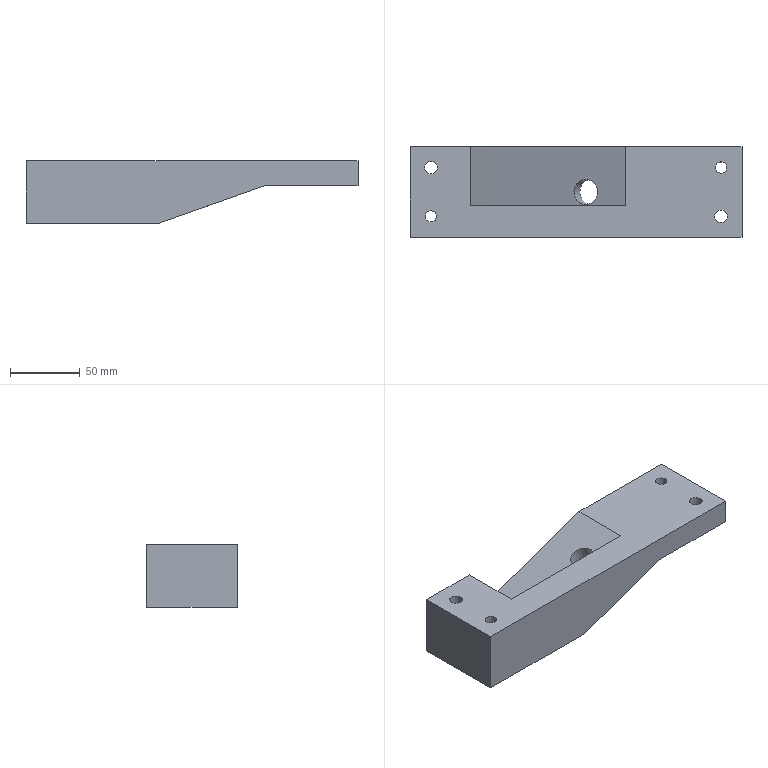Part | STEP file | HYDRAULIC-CYLINDER-BASE1_id474_x_t | 1 solid | 22 faces | box 238 x 65 x 45 mm | volume 410025 mm3 | plane 14 | cylinder 8 | commonest cylinder face diameters 8 x2 9 x2 14 x2 18 x1 31 x1
STEP:
#1=CARTESIAN_POINT('',(70.605,-50.,-302.095));
#2=VERTEX_POINT('',#1);
#3=CARTESIAN_POINT('',(85.215,-50.,-296.921));
#4=DIRECTION('',(0.3338,0.,-0.9426));
#5=DIRECTION('',(-0.9426,0.,-0.3338));
#6=AXIS2_PLACEMENT_3D('',#3,#4,#5);
#7=CIRCLE('',#6,15.5);
#8=EDGE_CURVE('',#2,#2,#7,.T.);
#9=ORIENTED_EDGE('',*,*,#8,.F.);
#10=EDGE_LOOP('',(#9));
#11=FACE_BOUND('',#10,.T.);
#12=CARTESIAN_POINT('',(73.943,-50.,-311.521));
#13=VERTEX_POINT('',#12);
#14=CARTESIAN_POINT('',(88.554,-50.,-306.347));
#15=DIRECTION('',(-0.3338,0.,0.9426));
#16=DIRECTION('',(-0.9426,0.,-0.3338));
#17=AXIS2_PLACEMENT_3D('',#14,#15,#16);
#18=CIRCLE('',#17,15.5);
#19=EDGE_CURVE('',#13,#13,#18,.T.);
#20=ORIENTED_EDGE('',*,*,#19,.F.);
#21=EDGE_LOOP('',(#20));
#22=FACE_BOUND('',#21,.T.);
#23=CARTESIAN_POINT('',(88.554,-50.,-306.347));
#24=DIRECTION('',(0.3338,0.,-0.9426));
#25=DIRECTION('',(-0.9426,0.,-0.3338));
#26=AXIS2_PLACEMENT_3D('',#23,#24,#25);
#27=CYLINDRICAL_SURFACE('',#26,15.5);
#28=ADVANCED_FACE('',(#11,#22),#27,.F.);
#29=CARTESIAN_POINT('',(76.732,-50.,-299.925));
#30=VERTEX_POINT('',#29);
#31=CARTESIAN_POINT('',(85.215,-50.,-296.921));
#32=DIRECTION('',(-0.3338,0.,0.9426));
#33=DIRECTION('',(-0.9426,0.,-0.3338));
#34=AXIS2_PLACEMENT_3D('',#31,#32,#33);
#35=CIRCLE('',#34,9.);
#36=EDGE_CURVE('',#30,#30,#35,.T.);
#37=ORIENTED_EDGE('',*,*,#36,.T.);
#38=EDGE_LOOP('',(#37));
#39=FACE_BOUND('',#38,.T.);
#40=ORIENTED_EDGE('',*,*,#8,.T.);
#41=EDGE_LOOP('',(#40));
#42=FACE_BOUND('',#41,.T.);
#43=CARTESIAN_POINT('',(-161.322,-82.5,-384.224));
#44=DIRECTION('',(0.3338,0.,-0.9426));
#45=DIRECTION('',(-0.9426,0.,-0.3338));
#46=AXIS2_PLACEMENT_3D('',#43,#44,#45);
#47=PLANE('',#46);
#48=ADVANCED_FACE('',(#39,#42),#47,.T.);
#49=CARTESIAN_POINT('',(-37.,-32.5,-311.));
#50=VERTEX_POINT('',#49);
#51=CARTESIAN_POINT('',(-30.,-32.5,-311.));
#52=DIRECTION('',(0.,0.,-1.));
#53=DIRECTION('',(-1.,0.,0.));
#54=AXIS2_PLACEMENT_3D('',#51,#52,#53);
#55=CIRCLE('',#54,7.);
#56=EDGE_CURVE('',#50,#50,#55,.T.);
#57=ORIENTED_EDGE('',*,*,#56,.F.);
#58=EDGE_LOOP('',(#57));
#59=FACE_BOUND('',#58,.T.);
#60=CARTESIAN_POINT('',(-37.,-32.5,-320.));
#61=VERTEX_POINT('',#60);
#62=CARTESIAN_POINT('',(-30.,-32.5,-320.));
#63=DIRECTION('',(0.,0.,1.));
#64=DIRECTION('',(-1.,0.,0.));
#65=AXIS2_PLACEMENT_3D('',#62,#63,#64);
#66=CIRCLE('',#65,7.);
#67=EDGE_CURVE('',#61,#61,#66,.T.);
#68=ORIENTED_EDGE('',*,*,#67,.F.);
#69=EDGE_LOOP('',(#68));
#70=FACE_BOUND('',#69,.T.);
#71=CARTESIAN_POINT('',(-30.,-32.5,-320.));
#72=DIRECTION('',(0.,0.,-1.));
#73=DIRECTION('',(-1.,0.,0.));
#74=AXIS2_PLACEMENT_3D('',#71,#72,#73);
#75=CYLINDRICAL_SURFACE('',#74,7.);
#76=ADVANCED_FACE('',(#59,#70),#75,.F.);
#77=CARTESIAN_POINT('',(171.,-67.5,-284.));
#78=VERTEX_POINT('',#77);
#79=CARTESIAN_POINT('',(178.,-67.5,-284.));
#80=DIRECTION('',(0.,0.,-1.));
#81=DIRECTION('',(-1.,0.,0.));
#82=AXIS2_PLACEMENT_3D('',#79,#80,#81);
#83=CIRCLE('',#82,7.);
#84=EDGE_CURVE('',#78,#78,#83,.T.);
#85=ORIENTED_EDGE('',*,*,#84,.F.);
#86=EDGE_LOOP('',(#85));
#87=FACE_BOUND('',#86,.T.);
#88=CARTESIAN_POINT('',(171.,-67.5,-293.));
#89=VERTEX_POINT('',#88);
#90=CARTESIAN_POINT('',(178.,-67.5,-293.));
#91=DIRECTION('',(0.,0.,1.));
#92=DIRECTION('',(-1.,0.,0.));
#93=AXIS2_PLACEMENT_3D('',#90,#91,#92);
#94=CIRCLE('',#93,7.);
#95=EDGE_CURVE('',#89,#89,#94,.T.);
#96=ORIENTED_EDGE('',*,*,#95,.F.);
#97=EDGE_LOOP('',(#96));
#98=FACE_BOUND('',#97,.T.);
#99=CARTESIAN_POINT('',(178.,-67.5,-293.));
#100=DIRECTION('',(0.,0.,-1.));
#101=DIRECTION('',(-1.,0.,0.));
#102=AXIS2_PLACEMENT_3D('',#99,#100,#101);
#103=CYLINDRICAL_SURFACE('',#102,7.);
#104=ADVANCED_FACE('',(#87,#98),#103,.F.);
#105=ORIENTED_EDGE('',*,*,#19,.T.);
#106=EDGE_LOOP('',(#105));
#107=FACE_BOUND('',#106,.T.);
#108=CARTESIAN_POINT('',(126.246,-82.5,-293.));
#109=VERTEX_POINT('',#108);
#110=CARTESIAN_POINT('',(126.246,-17.5,-293.));
#111=VERTEX_POINT('',#110);
#112=CARTESIAN_POINT('',(126.246,-82.5,-293.));
#113=DIRECTION('',(0.,1.,0.));
#114=VECTOR('',#113,1.);
#115=LINE('',#112,#114);
#116=EDGE_CURVE('',#109,#111,#115,.T.);
#117=ORIENTED_EDGE('',*,*,#116,.F.);
#118=CARTESIAN_POINT('',(50.,-82.5,-320.));
#119=VERTEX_POINT('',#118);
#120=CARTESIAN_POINT('',(126.246,-82.5,-293.));
#121=DIRECTION('',(-0.9426,0.,-0.3338));
#122=VECTOR('',#121,1.);
#123=LINE('',#120,#122);
#124=EDGE_CURVE('',#109,#119,#123,.T.);
#125=ORIENTED_EDGE('',*,*,#124,.T.);
#126=CARTESIAN_POINT('',(50.,-17.5,-320.));
#127=VERTEX_POINT('',#126);
#128=CARTESIAN_POINT('',(50.,-82.5,-320.));
#129=DIRECTION('',(0.,-1.,0.));
#130=VECTOR('',#129,1.);
#131=LINE('',#128,#130);
#132=EDGE_CURVE('',#127,#119,#131,.T.);
#133=ORIENTED_EDGE('',*,*,#132,.F.);
#134=CARTESIAN_POINT('',(126.246,-17.5,-293.));
#135=DIRECTION('',(-0.9426,0.,-0.3338));
#136=VECTOR('',#135,1.);
#137=LINE('',#134,#136);
#138=EDGE_CURVE('',#111,#127,#137,.T.);
#139=ORIENTED_EDGE('',*,*,#138,.F.);
#140=EDGE_LOOP('',(#117,#125,#133,#139));
#141=FACE_BOUND('',#140,.T.);
#142=CARTESIAN_POINT('',(126.246,-82.5,-293.));
#143=DIRECTION('',(0.3338,0.,-0.9426));
#144=DIRECTION('',(-0.9426,0.,-0.3338));
#145=AXIS2_PLACEMENT_3D('',#142,#143,#144);
#146=PLANE('',#145);
#147=ADVANCED_FACE('',(#107,#141),#146,.T.);
#148=ORIENTED_EDGE('',*,*,#36,.F.);
#149=EDGE_LOOP('',(#148));
#150=FACE_BOUND('',#149,.T.);
#151=CARTESIAN_POINT('',(72.541,-50.,-288.092));
#152=VERTEX_POINT('',#151);
#153=CARTESIAN_POINT('',(81.025,-50.,-285.088));
#154=DIRECTION('',(-0.3338,0.,0.9426));
#155=DIRECTION('',(-0.9426,0.,-0.3338));
#156=AXIS2_PLACEMENT_3D('',#153,#154,#155);
#157=CIRCLE('',#156,9.);
#158=EDGE_CURVE('',#152,#152,#157,.T.);
#159=ORIENTED_EDGE('',*,*,#158,.T.);
#160=EDGE_LOOP('',(#159));
#161=FACE_BOUND('',#160,.T.);
#162=CARTESIAN_POINT('',(88.554,-50.,-306.347));
#163=DIRECTION('',(0.3338,0.,-0.9426));
#164=DIRECTION('',(-0.9426,0.,-0.3338));
#165=AXIS2_PLACEMENT_3D('',#162,#163,#164);
#166=CYLINDRICAL_SURFACE('',#165,9.);
#167=ADVANCED_FACE('',(#150,#161),#166,.F.);
#168=CARTESIAN_POINT('',(-34.5,-32.5,-311.));
#169=VERTEX_POINT('',#168);
#170=CARTESIAN_POINT('',(-30.,-32.5,-311.));
#171=DIRECTION('',(0.,0.,1.));
#172=DIRECTION('',(-1.,0.,0.));
#173=AXIS2_PLACEMENT_3D('',#170,#171,#172);
#174=CIRCLE('',#173,4.5);
#175=EDGE_CURVE('',#169,#169,#174,.T.);
#176=ORIENTED_EDGE('',*,*,#175,.T.);
#177=EDGE_LOOP('',(#176));
#178=FACE_BOUND('',#177,.T.);
#179=ORIENTED_EDGE('',*,*,#56,.T.);
#180=EDGE_LOOP('',(#179));
#181=FACE_BOUND('',#180,.T.);
#182=CARTESIAN_POINT('',(-200.,-82.5,-311.));
#183=DIRECTION('',(0.,0.,-1.));
#184=DIRECTION('',(-1.,0.,0.));
#185=AXIS2_PLACEMENT_3D('',#182,#183,#184);
#186=PLANE('',#185);
#187=ADVANCED_FACE('',(#178,#181),#186,.T.);
#188=ORIENTED_EDGE('',*,*,#67,.T.);
#189=EDGE_LOOP('',(#188));
#190=FACE_BOUND('',#189,.T.);
#191=CARTESIAN_POINT('',(-34.,-67.5,-320.));
#192=VERTEX_POINT('',#191);
#193=CARTESIAN_POINT('',(-30.,-67.5,-320.));
#194=DIRECTION('',(0.,0.,1.));
#195=DIRECTION('',(-1.,0.,0.));
#196=AXIS2_PLACEMENT_3D('',#193,#194,#195);
#197=CIRCLE('',#196,4.);
#198=EDGE_CURVE('',#192,#192,#197,.T.);
#199=ORIENTED_EDGE('',*,*,#198,.T.);
#200=EDGE_LOOP('',(#199));
#201=FACE_BOUND('',#200,.T.);
#202=ORIENTED_EDGE('',*,*,#132,.T.);
#203=CARTESIAN_POINT('',(-45.,-82.5,-320.));
#204=VERTEX_POINT('',#203);
#205=CARTESIAN_POINT('',(-200.,-82.5,-320.));
#206=DIRECTION('',(-1.,0.,0.));
#207=VECTOR('',#206,1.);
#208=LINE('',#205,#207);
#209=EDGE_CURVE('',#119,#204,#208,.T.);
#210=ORIENTED_EDGE('',*,*,#209,.T.);
#211=CARTESIAN_POINT('',(-45.,-17.5,-320.));
#212=VERTEX_POINT('',#211);
#213=CARTESIAN_POINT('',(-45.,-82.5,-320.));
#214=DIRECTION('',(0.,-1.,0.));
#215=VECTOR('',#214,1.);
#216=LINE('',#213,#215);
#217=EDGE_CURVE('',#212,#204,#216,.T.);
#218=ORIENTED_EDGE('',*,*,#217,.F.);
#219=CARTESIAN_POINT('',(-200.,-17.5,-320.));
#220=DIRECTION('',(-1.,0.,0.));
#221=VECTOR('',#220,1.);
#222=LINE('',#219,#221);
#223=EDGE_CURVE('',#127,#212,#222,.T.);
#224=ORIENTED_EDGE('',*,*,#223,.F.);
#225=EDGE_LOOP('',(#202,#210,#218,#224));
#226=FACE_BOUND('',#225,.T.);
#227=CARTESIAN_POINT('',(50.,-82.5,-320.));
#228=DIRECTION('',(0.,0.,-1.));
#229=DIRECTION('',(-1.,0.,0.));
#230=AXIS2_PLACEMENT_3D('',#227,#228,#229);
#231=PLANE('',#230);
#232=ADVANCED_FACE('',(#190,#201,#226),#231,.T.);
#233=CARTESIAN_POINT('',(173.5,-67.5,-284.));
#234=VERTEX_POINT('',#233);
#235=CARTESIAN_POINT('',(178.,-67.5,-284.));
#236=DIRECTION('',(0.,0.,1.));
#237=DIRECTION('',(-1.,0.,0.));
#238=AXIS2_PLACEMENT_3D('',#235,#236,#237);
#239=CIRCLE('',#238,4.5);
#240=EDGE_CURVE('',#234,#234,#239,.T.);
#241=ORIENTED_EDGE('',*,*,#240,.T.);
#242=EDGE_LOOP('',(#241));
#243=FACE_BOUND('',#242,.T.);
#244=ORIENTED_EDGE('',*,*,#84,.T.);
#245=EDGE_LOOP('',(#244));
#246=FACE_BOUND('',#245,.T.);
#247=CARTESIAN_POINT('',(-200.,-82.5,-284.));
#248=DIRECTION('',(0.,0.,-1.));
#249=DIRECTION('',(-1.,0.,0.));
#250=AXIS2_PLACEMENT_3D('',#247,#248,#249);
#251=PLANE('',#250);
#252=ADVANCED_FACE('',(#243,#246),#251,.T.);
#253=ORIENTED_EDGE('',*,*,#95,.T.);
#254=EDGE_LOOP('',(#253));
#255=FACE_BOUND('',#254,.T.);
#256=CARTESIAN_POINT('',(174.,-32.5,-293.));
#257=VERTEX_POINT('',#256);
#258=CARTESIAN_POINT('',(178.,-32.5,-293.));
#259=DIRECTION('',(0.,0.,1.));
#260=DIRECTION('',(-1.,0.,0.));
#261=AXIS2_PLACEMENT_3D('',#258,#259,#260);
#262=CIRCLE('',#261,4.);
#263=EDGE_CURVE('',#257,#257,#262,.T.);
#264=ORIENTED_EDGE('',*,*,#263,.T.);
#265=EDGE_LOOP('',(#264));
#266=FACE_BOUND('',#265,.T.);
#267=CARTESIAN_POINT('',(193.,-82.5,-293.));
#268=VERTEX_POINT('',#267);
#269=CARTESIAN_POINT('',(193.,-17.5,-293.));
#270=VERTEX_POINT('',#269);
#271=CARTESIAN_POINT('',(193.,-82.5,-293.));
#272=DIRECTION('',(0.,1.,0.));
#273=VECTOR('',#272,1.);
#274=LINE('',#271,#273);
#275=EDGE_CURVE('',#268,#270,#274,.T.);
#276=ORIENTED_EDGE('',*,*,#275,.F.);
#277=CARTESIAN_POINT('',(-200.,-82.5,-293.));
#278=DIRECTION('',(-1.,0.,0.));
#279=VECTOR('',#278,1.);
#280=LINE('',#277,#279);
#281=EDGE_CURVE('',#268,#109,#280,.T.);
#282=ORIENTED_EDGE('',*,*,#281,.T.);
#283=ORIENTED_EDGE('',*,*,#116,.T.);
#284=CARTESIAN_POINT('',(-200.,-17.5,-293.));
#285=DIRECTION('',(-1.,0.,0.));
#286=VECTOR('',#285,1.);
#287=LINE('',#284,#286);
#288=EDGE_CURVE('',#270,#111,#287,.T.);
#289=ORIENTED_EDGE('',*,*,#288,.F.);
#290=EDGE_LOOP('',(#276,#282,#283,#289));
#291=FACE_BOUND('',#290,.T.);
#292=CARTESIAN_POINT('',(193.,-82.5,-293.));
#293=DIRECTION('',(0.,0.,-1.));
#294=DIRECTION('',(-1.,0.,0.));
#295=AXIS2_PLACEMENT_3D('',#292,#293,#294);
#296=PLANE('',#295);
#297=ADVANCED_FACE('',(#255,#266,#291),#296,.T.);
#298=CARTESIAN_POINT('',(10.798,-60.,-309.957));
#299=VERTEX_POINT('',#298);
#300=CARTESIAN_POINT('',(-1.58,-60.,-275.));
#301=VERTEX_POINT('',#300);
#302=CARTESIAN_POINT('',(10.798,-60.,-309.957));
#303=DIRECTION('',(-0.3338,0.,0.9426));
#304=VECTOR('',#303,1.);
#305=LINE('',#302,#304);
#306=EDGE_CURVE('',#299,#301,#305,.T.);
#307=ORIENTED_EDGE('',*,*,#306,.F.);
#308=CARTESIAN_POINT('',(10.798,-17.5,-309.957));
#309=VERTEX_POINT('',#308);
#310=CARTESIAN_POINT('',(10.798,-17.5,-309.957));
#311=DIRECTION('',(0.,1.,0.));
#312=VECTOR('',#311,1.);
#313=LINE('',#310,#312);
#314=EDGE_CURVE('',#299,#309,#313,.T.);
#315=ORIENTED_EDGE('',*,*,#314,.T.);
#316=CARTESIAN_POINT('',(-1.58,-17.5,-275.));
#317=VERTEX_POINT('',#316);
#318=CARTESIAN_POINT('',(-1.58,-17.5,-275.));
#319=DIRECTION('',(0.3338,0.,-0.9426));
#320=VECTOR('',#319,1.);
#321=LINE('',#318,#320);
#322=EDGE_CURVE('',#317,#309,#321,.T.);
#323=ORIENTED_EDGE('',*,*,#322,.F.);
#324=CARTESIAN_POINT('',(-1.58,-82.5,-275.));
#325=DIRECTION('',(0.,1.,0.));
#326=VECTOR('',#325,1.);
#327=LINE('',#324,#326);
#328=EDGE_CURVE('',#301,#317,#327,.T.);
#329=ORIENTED_EDGE('',*,*,#328,.F.);
#330=EDGE_LOOP('',(#307,#315,#323,#329));
#331=FACE_OUTER_BOUND('',#330,.T.);
#332=CARTESIAN_POINT('',(10.798,-17.5,-309.957));
#333=DIRECTION('',(-0.9426,0.,-0.3338));
#334=DIRECTION('',(-0.3338,0.,0.9426));
#335=AXIS2_PLACEMENT_3D('',#332,#333,#334);
#336=PLANE('',#335);
#337=ADVANCED_FACE('',(#331),#336,.F.);
#338=ORIENTED_EDGE('',*,*,#217,.T.);
#339=CARTESIAN_POINT('',(-45.,-82.5,-275.));
#340=VERTEX_POINT('',#339);
#341=CARTESIAN_POINT('',(-45.,-82.5,-275.));
#342=DIRECTION('',(0.,0.,1.));
#343=VECTOR('',#342,1.);
#344=LINE('',#341,#343);
#345=EDGE_CURVE('',#204,#340,#344,.T.);
#346=ORIENTED_EDGE('',*,*,#345,.T.);
#347=CARTESIAN_POINT('',(-45.,-17.5,-275.));
#348=VERTEX_POINT('',#347);
#349=CARTESIAN_POINT('',(-45.,-82.5,-275.));
#350=DIRECTION('',(0.,-1.,0.));
#351=VECTOR('',#350,1.);
#352=LINE('',#349,#351);
#353=EDGE_CURVE('',#348,#340,#352,.T.);
#354=ORIENTED_EDGE('',*,*,#353,.F.);
#355=CARTESIAN_POINT('',(-45.,-17.5,-275.));
#356=DIRECTION('',(0.,0.,1.));
#357=VECTOR('',#356,1.);
#358=LINE('',#355,#357);
#359=EDGE_CURVE('',#212,#348,#358,.T.);
#360=ORIENTED_EDGE('',*,*,#359,.F.);
#361=EDGE_LOOP('',(#338,#346,#354,#360));
#362=FACE_OUTER_BOUND('',#361,.T.);
#363=CARTESIAN_POINT('',(-45.,-82.5,-320.));
#364=DIRECTION('',(-1.,0.,0.));
#365=DIRECTION('',(0.,0.,1.));
#366=AXIS2_PLACEMENT_3D('',#363,#364,#365);
#367=PLANE('',#366);
#368=ADVANCED_FACE('',(#362),#367,.T.);
#369=ORIENTED_EDGE('',*,*,#124,.F.);
#370=ORIENTED_EDGE('',*,*,#281,.F.);
#371=CARTESIAN_POINT('',(193.,-82.5,-275.));
#372=VERTEX_POINT('',#371);
#373=CARTESIAN_POINT('',(193.,-82.5,-275.));
#374=DIRECTION('',(0.,0.,-1.));
#375=VECTOR('',#374,1.);
#376=LINE('',#373,#375);
#377=EDGE_CURVE('',#372,#268,#376,.T.);
#378=ORIENTED_EDGE('',*,*,#377,.F.);
#379=CARTESIAN_POINT('',(-45.,-82.5,-275.));
#380=DIRECTION('',(1.,0.,0.));
#381=VECTOR('',#380,1.);
#382=LINE('',#379,#381);
#383=EDGE_CURVE('',#340,#372,#382,.T.);
#384=ORIENTED_EDGE('',*,*,#383,.F.);
#385=ORIENTED_EDGE('',*,*,#345,.F.);
#386=ORIENTED_EDGE('',*,*,#209,.F.);
#387=EDGE_LOOP('',(#369,#370,#378,#384,#385,#386));
#388=FACE_OUTER_BOUND('',#387,.T.);
#389=CARTESIAN_POINT('',(-200.,-82.5,-275.));
#390=DIRECTION('',(0.,1.,0.));
#391=DIRECTION('',(0.,0.,1.));
#392=AXIS2_PLACEMENT_3D('',#389,#390,#391);
#393=PLANE('',#392);
#394=ADVANCED_FACE('',(#388),#393,.F.);
#395=CARTESIAN_POINT('',(193.,-17.5,-275.));
#396=VERTEX_POINT('',#395);
#397=CARTESIAN_POINT('',(193.,-82.5,-275.));
#398=DIRECTION('',(0.,1.,0.));
#399=VECTOR('',#398,1.);
#400=LINE('',#397,#399);
#401=EDGE_CURVE('',#372,#396,#400,.T.);
#402=ORIENTED_EDGE('',*,*,#401,.F.);
#403=ORIENTED_EDGE('',*,*,#377,.T.);
#404=ORIENTED_EDGE('',*,*,#275,.T.);
#405=CARTESIAN_POINT('',(193.,-17.5,-275.));
#406=DIRECTION('',(0.,0.,-1.));
#407=VECTOR('',#406,1.);
#408=LINE('',#405,#407);
#409=EDGE_CURVE('',#396,#270,#408,.T.);
#410=ORIENTED_EDGE('',*,*,#409,.F.);
#411=EDGE_LOOP('',(#402,#403,#404,#410));
#412=FACE_OUTER_BOUND('',#411,.T.);
#413=CARTESIAN_POINT('',(193.,-82.5,-275.));
#414=DIRECTION('',(1.,0.,0.));
#415=DIRECTION('',(0.,0.,-1.));
#416=AXIS2_PLACEMENT_3D('',#413,#414,#415);
#417=PLANE('',#416);
#418=ADVANCED_FACE('',(#412),#417,.T.);
#419=CARTESIAN_POINT('',(-45.,-17.5,-275.));
#420=DIRECTION('',(-1.,0.,0.));
#421=VECTOR('',#420,1.);
#422=LINE('',#419,#421);
#423=EDGE_CURVE('',#317,#348,#422,.T.);
#424=ORIENTED_EDGE('',*,*,#423,.F.);
#425=ORIENTED_EDGE('',*,*,#322,.T.);
#426=CARTESIAN_POINT('',(109.513,-17.5,-275.));
#427=VERTEX_POINT('',#426);
#428=CARTESIAN_POINT('',(109.513,-17.5,-275.));
#429=DIRECTION('',(0.9426,0.,0.3338));
#430=VECTOR('',#429,1.);
#431=LINE('',#428,#430);
#432=EDGE_CURVE('',#309,#427,#431,.T.);
#433=ORIENTED_EDGE('',*,*,#432,.T.);
#434=CARTESIAN_POINT('',(-45.,-17.5,-275.));
#435=DIRECTION('',(-1.,0.,0.));
#436=VECTOR('',#435,1.);
#437=LINE('',#434,#436);
#438=EDGE_CURVE('',#396,#427,#437,.T.);
#439=ORIENTED_EDGE('',*,*,#438,.F.);
#440=ORIENTED_EDGE('',*,*,#409,.T.);
#441=ORIENTED_EDGE('',*,*,#288,.T.);
#442=ORIENTED_EDGE('',*,*,#138,.T.);
#443=ORIENTED_EDGE('',*,*,#223,.T.);
#444=ORIENTED_EDGE('',*,*,#359,.T.);
#445=EDGE_LOOP('',(#424,#425,#433,#439,#440,#441,#442,#443,#444));
#446=FACE_OUTER_BOUND('',#445,.T.);
#447=CARTESIAN_POINT('',(-200.,-17.5,-275.));
#448=DIRECTION('',(0.,1.,0.));
#449=DIRECTION('',(0.,0.,1.));
#450=AXIS2_PLACEMENT_3D('',#447,#448,#449);
#451=PLANE('',#450);
#452=ADVANCED_FACE('',(#446),#451,.T.);
#453=ORIENTED_EDGE('',*,*,#158,.F.);
#454=EDGE_LOOP('',(#453));
#455=FACE_BOUND('',#454,.T.);
#456=CARTESIAN_POINT('',(109.513,-60.,-275.));
#457=VERTEX_POINT('',#456);
#458=CARTESIAN_POINT('',(109.513,-60.,-275.));
#459=DIRECTION('',(-0.9426,0.,-0.3338));
#460=VECTOR('',#459,1.);
#461=LINE('',#458,#460);
#462=EDGE_CURVE('',#457,#299,#461,.T.);
#463=ORIENTED_EDGE('',*,*,#462,.F.);
#464=CARTESIAN_POINT('',(109.513,-82.5,-275.));
#465=DIRECTION('',(0.,-1.,0.));
#466=VECTOR('',#465,1.);
#467=LINE('',#464,#466);
#468=EDGE_CURVE('',#427,#457,#467,.T.);
#469=ORIENTED_EDGE('',*,*,#468,.F.);
#470=ORIENTED_EDGE('',*,*,#432,.F.);
#471=ORIENTED_EDGE('',*,*,#314,.F.);
#472=EDGE_LOOP('',(#463,#469,#470,#471));
#473=FACE_BOUND('',#472,.T.);
#474=CARTESIAN_POINT('',(109.513,-17.5,-275.));
#475=DIRECTION('',(0.3338,0.,-0.9426));
#476=DIRECTION('',(-0.9426,0.,-0.3338));
#477=AXIS2_PLACEMENT_3D('',#474,#475,#476);
#478=PLANE('',#477);
#479=ADVANCED_FACE('',(#455,#473),#478,.F.);
#480=ORIENTED_EDGE('',*,*,#306,.T.);
#481=CARTESIAN_POINT('',(-45.,-60.,-275.));
#482=DIRECTION('',(-1.,0.,0.));
#483=VECTOR('',#482,1.);
#484=LINE('',#481,#483);
#485=EDGE_CURVE('',#457,#301,#484,.T.);
#486=ORIENTED_EDGE('',*,*,#485,.F.);
#487=ORIENTED_EDGE('',*,*,#462,.T.);
#488=EDGE_LOOP('',(#480,#486,#487));
#489=FACE_OUTER_BOUND('',#488,.T.);
#490=CARTESIAN_POINT('',(50.,-60.,-320.));
#491=DIRECTION('',(0.,1.,0.));
#492=DIRECTION('',(0.,0.,1.));
#493=AXIS2_PLACEMENT_3D('',#490,#491,#492);
#494=PLANE('',#493);
#495=ADVANCED_FACE('',(#489),#494,.T.);
#496=CARTESIAN_POINT('',(-34.5,-32.5,-275.));
#497=VERTEX_POINT('',#496);
#498=CARTESIAN_POINT('',(-30.,-32.5,-275.));
#499=DIRECTION('',(0.,0.,-1.));
#500=DIRECTION('',(-1.,0.,0.));
#501=AXIS2_PLACEMENT_3D('',#498,#499,#500);
#502=CIRCLE('',#501,4.5);
#503=EDGE_CURVE('',#497,#497,#502,.T.);
#504=ORIENTED_EDGE('',*,*,#503,.F.);
#505=EDGE_LOOP('',(#504));
#506=FACE_BOUND('',#505,.T.);
#507=ORIENTED_EDGE('',*,*,#175,.F.);
#508=EDGE_LOOP('',(#507));
#509=FACE_BOUND('',#508,.T.);
#510=CARTESIAN_POINT('',(-30.,-32.5,-320.));
#511=DIRECTION('',(0.,0.,-1.));
#512=DIRECTION('',(-1.,0.,0.));
#513=AXIS2_PLACEMENT_3D('',#510,#511,#512);
#514=CYLINDRICAL_SURFACE('',#513,4.5);
#515=ADVANCED_FACE('',(#506,#509),#514,.F.);
#516=ORIENTED_EDGE('',*,*,#198,.F.);
#517=EDGE_LOOP('',(#516));
#518=FACE_BOUND('',#517,.T.);
#519=CARTESIAN_POINT('',(-34.,-67.5,-275.));
#520=VERTEX_POINT('',#519);
#521=CARTESIAN_POINT('',(-30.,-67.5,-275.));
#522=DIRECTION('',(0.,0.,-1.));
#523=DIRECTION('',(-1.,0.,0.));
#524=AXIS2_PLACEMENT_3D('',#521,#522,#523);
#525=CIRCLE('',#524,4.);
#526=EDGE_CURVE('',#520,#520,#525,.T.);
#527=ORIENTED_EDGE('',*,*,#526,.F.);
#528=EDGE_LOOP('',(#527));
#529=FACE_BOUND('',#528,.T.);
#530=CARTESIAN_POINT('',(-30.,-67.5,-320.));
#531=DIRECTION('',(0.,0.,-1.));
#532=DIRECTION('',(-1.,0.,0.));
#533=AXIS2_PLACEMENT_3D('',#530,#531,#532);
#534=CYLINDRICAL_SURFACE('',#533,4.);
#535=ADVANCED_FACE('',(#518,#529),#534,.F.);
#536=CARTESIAN_POINT('',(173.5,-67.5,-275.));
#537=VERTEX_POINT('',#536);
#538=CARTESIAN_POINT('',(178.,-67.5,-275.));
#539=DIRECTION('',(0.,0.,-1.));
#540=DIRECTION('',(-1.,0.,0.));
#541=AXIS2_PLACEMENT_3D('',#538,#539,#540);
#542=CIRCLE('',#541,4.5);
#543=EDGE_CURVE('',#537,#537,#542,.T.);
#544=ORIENTED_EDGE('',*,*,#543,.F.);
#545=EDGE_LOOP('',(#544));
#546=FACE_BOUND('',#545,.T.);
#547=ORIENTED_EDGE('',*,*,#240,.F.);
#548=EDGE_LOOP('',(#547));
#549=FACE_BOUND('',#548,.T.);
#550=CARTESIAN_POINT('',(178.,-67.5,-320.));
#551=DIRECTION('',(0.,0.,-1.));
#552=DIRECTION('',(-1.,0.,0.));
#553=AXIS2_PLACEMENT_3D('',#550,#551,#552);
#554=CYLINDRICAL_SURFACE('',#553,4.5);
#555=ADVANCED_FACE('',(#546,#549),#554,.F.);
#556=ORIENTED_EDGE('',*,*,#263,.F.);
#557=EDGE_LOOP('',(#556));
#558=FACE_BOUND('',#557,.T.);
#559=CARTESIAN_POINT('',(174.,-32.5,-275.));
#560=VERTEX_POINT('',#559);
#561=CARTESIAN_POINT('',(178.,-32.5,-275.));
#562=DIRECTION('',(0.,0.,-1.));
#563=DIRECTION('',(-1.,0.,0.));
#564=AXIS2_PLACEMENT_3D('',#561,#562,#563);
#565=CIRCLE('',#564,4.);
#566=EDGE_CURVE('',#560,#560,#565,.T.);
#567=ORIENTED_EDGE('',*,*,#566,.F.);
#568=EDGE_LOOP('',(#567));
#569=FACE_BOUND('',#568,.T.);
#570=CARTESIAN_POINT('',(178.,-32.5,-320.));
#571=DIRECTION('',(0.,0.,-1.));
#572=DIRECTION('',(-1.,0.,0.));
#573=AXIS2_PLACEMENT_3D('',#570,#571,#572);
#574=CYLINDRICAL_SURFACE('',#573,4.);
#575=ADVANCED_FACE('',(#558,#569),#574,.F.);
#576=ORIENTED_EDGE('',*,*,#566,.T.);
#577=EDGE_LOOP('',(#576));
#578=FACE_BOUND('',#577,.T.);
#579=ORIENTED_EDGE('',*,*,#543,.T.);
#580=EDGE_LOOP('',(#579));
#581=FACE_BOUND('',#580,.T.);
#582=ORIENTED_EDGE('',*,*,#526,.T.);
#583=EDGE_LOOP('',(#582));
#584=FACE_BOUND('',#583,.T.);
#585=ORIENTED_EDGE('',*,*,#503,.T.);
#586=EDGE_LOOP('',(#585));
#587=FACE_BOUND('',#586,.T.);
#588=ORIENTED_EDGE('',*,*,#468,.T.);
#589=ORIENTED_EDGE('',*,*,#485,.T.);
#590=ORIENTED_EDGE('',*,*,#328,.T.);
#591=ORIENTED_EDGE('',*,*,#423,.T.);
#592=ORIENTED_EDGE('',*,*,#353,.T.);
#593=ORIENTED_EDGE('',*,*,#383,.T.);
#594=ORIENTED_EDGE('',*,*,#401,.T.);
#595=ORIENTED_EDGE('',*,*,#438,.T.);
#596=EDGE_LOOP('',(#588,#589,#590,#591,#592,#593,#594,#595));
#597=FACE_BOUND('',#596,.T.);
#598=CARTESIAN_POINT('',(-45.,-82.5,-275.));
#599=DIRECTION('',(0.,0.,1.));
#600=DIRECTION('',(1.,0.,0.));
#601=AXIS2_PLACEMENT_3D('',#598,#599,#600);
#602=PLANE('',#601);
#603=ADVANCED_FACE('',(#578,#581,#584,#587,#597),#602,.T.);
#604=CLOSED_SHELL('',(#28,#48,#76,#104,#147,#167,#187,#232,#252,#297,#337,#368,#394,#418,#452,#479,#495,#515,#535,#555,#575,#603));
#605=MANIFOLD_SOLID_BREP('',#604);
#606=(LENGTH_UNIT()NAMED_UNIT(*)SI_UNIT(.MILLI.,.METRE.));
#607=UNCERTAINTY_MEASURE_WITH_UNIT(LENGTH_MEASURE(0.00002),#606,'','');
#608=(NAMED_UNIT(*)PLANE_ANGLE_UNIT()SI_UNIT($,.RADIAN.));
#609=PLANE_ANGLE_MEASURE_WITH_UNIT(PLANE_ANGLE_MEASURE(0.01745),#608);
#610=DIMENSIONAL_EXPONENTS(0.,0.,0.,0.,0.,0.,0.);
#611=(CONVERSION_BASED_UNIT('DEGREE',#609)NAMED_UNIT(#610)PLANE_ANGLE_UNIT());
#612=(NAMED_UNIT(*)SI_UNIT($,.STERADIAN.)SOLID_ANGLE_UNIT());
#613=(GEOMETRIC_REPRESENTATION_CONTEXT(3)GLOBAL_UNCERTAINTY_ASSIGNED_CONTEXT((#607))GLOBAL_UNIT_ASSIGNED_CONTEXT((#606,#611,#612))REPRESENTATION_CONTEXT('',''));
#614=ADVANCED_BREP_SHAPE_REPRESENTATION('',(#605),#613);